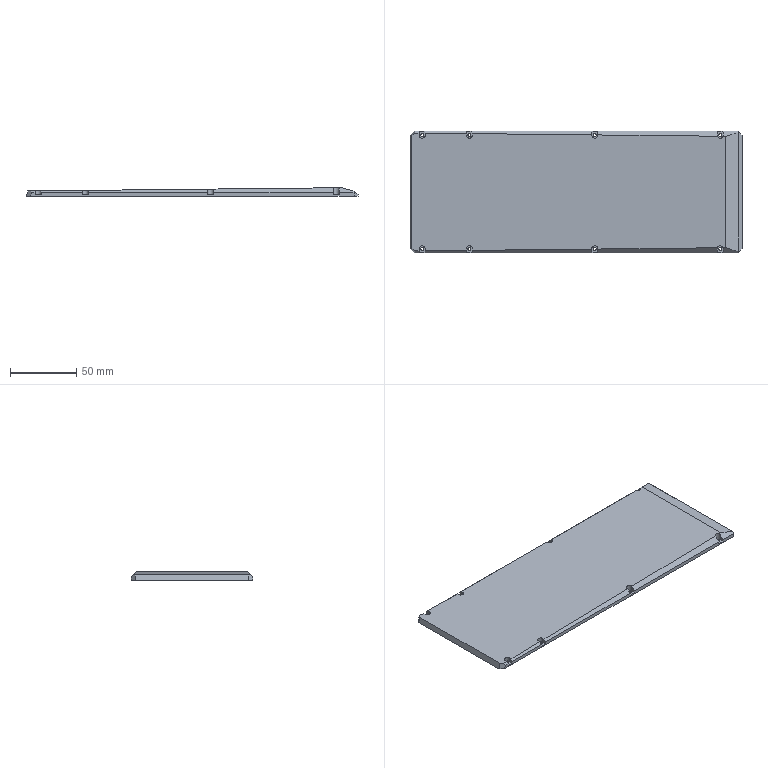CAM job | NX | 3-axis milling, drilling | part box 251.5 x 92 x 6.5 mm | stock box 260 x 100 x 10 mm
Tools:
number,name,description,diameter,corner_radius,flute_length,length,flutes
2,D2-6-D4-50-3T-ROUGH,D2-6-D4-50-3T-粗,2.0,0.0,6.0,7.0,2
0,D3-9-D4-50-3T-ROUGH,D3-9-D4-50-3T,3.0,0.0,9.0,10.0,3
0,D3-9-D4-50-3T-FINISH,D3-9-D4-50-3T-精,3.0,0.0,9.0,10.0,2
3,D6-18-D6-50-3T-FINISH,D6-18-D6-50-3T,6.0,0.0,18.0,50.0,3
1,D10-30-D10-75-3T-ROUGH,D10-30-D10-75-3T-粗,10.0,0.0,30.0,75.0,2
1,D12-36-D12-120-3TFINISH,D12-55-D12-120-3T,12.0,0.0,55.0,120.0,3
13,D50FACEMILL,D50面刀,50.0,0.0,30.0,30.0,4
11,D63FACEMILL,D63面刀,63.0,0.0,30.0,30.0,4
3,DRILLD1.84-11-D3-40,钻刀D1.84-11-D3-40,1.84,0.0,11.0,12.0,2
5,DRILLD2.4-35-61,钻刀D2.5-35-61,2.4,0.0,36.0,61.0,2
5,FORMTAPM2-12-D3-39,挤压M2-12-D3-39,2.0,0.0,12.5,14.5,2
4,CHAMFERD4-90DEG,倒角D4-90度,4.0,0.0,5.0,50.0,2
12,D4R0.5,Milling Tool-5 Parameters,4.0,0.5,50.0,75.0,2
Operations:
program,operation,operation_type,tool,method,geometry_group,spindle_rpm,surface_speed,feed_per_tooth,feed_cut,feed_plunge,cut_length_mm,path_length_mm,cut_time_min,machine_time_min
A1,PLANAR_MILL_4,PlanarMilling,D63FACEMILL,METHOD,A-G54,3500.0,692.0,0.0571,800.0,100.0,657.0,1096.483,0.8213,0.8652
A1,PLANAR_MILL,PlanarMilling,D10-30-D10-75-3T-ROUGH,METHOD,WORKPIECE_54,4500.0,141.0,0.1667,1500.0,100.0,8744.461,9081.313,5.83,5.863
A1,PLANAR_MILL_COPY_1,PlanarMilling,D10-30-D10-75-3T-ROUGH,METHOD,WORKPIECE_54,4500.0,141.0,0.1667,1500.0,100.0,4614.076,4868.443,3.076,3.102
A1,PLANAR_PROFILING,PlanarMilling,D10-30-D10-75-3T-ROUGH,METHOD,WORKPIECE_54,4500.0,141.0,0.1111,1000.0,100.0,5055.326,5144.065,5.055,5.064
A1,PLANAR_MILL_COPY_COPY,PlanarMilling,D6-18-D6-50-3T-FINISH,METHOD,WORKPIECE_54,4000.0,75.0,0.0667,800.0,100.0,69.184,577.146,0.0865,0.1373
A1,PLANAR_MILL_COPY_COPY_COPY_1,PlanarMilling,D6-18-D6-50-3T-FINISH,METHOD,WORKPIECE_54,4000.0,75.0,0.0667,800.0,100.0,34.592,216.179,0.0432,0.0614
A1,PLANAR_MILL_COPY,PlanarMilling,D6-18-D6-50-3T-FINISH,METHOD,WORKPIECE_54,4000.0,125.0,0.0667,800.0,100.0,1137.2,1194.6,1.421,1.427
A1,PLANAR_MILL_COPY_COPY_1,PlanarMilling,D6-18-D6-50-3T-FINISH,METHOD,WORKPIECE_54,4000.0,125.0,0.0667,800.0,100.0,2620.054,2682.454,3.275,3.281
A1,PLANAR_MILL_1,PlanarMilling,D6-18-D6-50-3T-FINISH,METHOD,WORKPIECE_54,4000.0,125.0,0.0667,800.0,100.0,710.995,780.995,0.8887,0.8957
A1,PLANAR_MILL_COPY_COPY_COPY,PlanarMilling,D6-18-D6-50-3T-FINISH,METHOD,WORKPIECE_54,4000.0,75.0,0.0667,800.0,100.0,448.283,510.683,0.5604,0.5666
A1,PLANAR_MILL_COPY_COPY_COPY_1_COPY,PlanarMilling,D6-18-D6-50-3T-FINISH,METHOD,WORKPIECE_54,4000.0,75.0,0.0667,800.0,100.0,216.283,275.683,0.2704,0.2763
A1,PLANAR_MILL_5,PlanarMilling,D6-18-D6-50-3T-FINISH,METHOD,A-G54,6500.0,122.0,0.041,800.0,100.0,740.395,1024.154,0.9255,0.9539
A1,PLANAR_MILL_5_COPY,PlanarMilling,D6-18-D6-50-3T-FINISH,METHOD,A-G54,6500.0,122.0,0.041,800.0,100.0,185.899,251.499,0.2324,0.2389
A1,平面铣倒角,PlanarMilling,CHAMFERD4-90DEG,METHOD,WORKPIECE_54,3500.0,43.0,0.1429,1000.0,100.0,585.85,641.85,0.5859,0.5915
A1,PLANAR_MILL_5_COPY_COPY,PlanarMilling,CHAMFERD4-90DEG,METHOD,A-G54,4500.0,56.0,0.0667,600.0,100.0,193.876,259.076,0.3231,0.3296
A1,平面铣倒角_COPY,PlanarMilling,CHAMFERD4-90DEG,METHOD,WORKPIECE_54,3500.0,43.0,0.1429,1000.0,100.0,81.284,139.684,0.0813,0.0871
A1,平面铣倒角_1,PlanarMilling,CHAMFERD4-90DEG,METHOD,WORKPIECE_54,3500.0,43.0,0.1429,1000.0,100.0,696.845,754.845,0.6968,0.7026
A1,DRILLING,Operation,CHAMFERD4-90DEG,METHOD,WORKPIECE_54,3000.0,37.0,0.025,150.0,0.0,34.0,1169.84,0.2267,0.3403
A1,DRILLING_COPY,Operation,DRILLD2.4-35-61,METHOD,WORKPIECE_54,3000.0,22.0,0.0333,200.0,0.0,72.0,1245.84,0.36,0.4774
B1,ADAPTIVE_MILLING,CavityMilling,D10-30-D10-75-3T-ROUGH,METHOD,WORKPIECE_55,6500.0,204.0,0.2308,3000.0,100.0,59868.173,68596.254,13.506,14.379
B1,CURVE_DRIVE_COPY,SurfaceContour,D4R0.5,METHOD,B-G55,6000.0,188.0,0.25,3000.0,100.0,20608.91,20984.951,6.87,6.907
B1,CURVE_DRIVE_COPY_COPY,SurfaceContour,D4R0.5,METHOD,B-G55,6000.0,188.0,0.25,3000.0,100.0,21012.824,22542.308,7.004,7.157
B1,CURVE_DRIVE_COPY_COPY_COPY,SurfaceContour,D4R0.5,METHOD,B-G55,6000.0,188.0,0.25,3000.0,100.0,473.306,685.412,0.1578,0.179
C1,FLOOR_FACING_1,VolumeBased25DMillingOperation,D50FACEMILL,METHOD,C-G56,3000.0,100.0,0.1178,800.0,100.0,930.818,984.718,1.163,1.169
C1,FLOOR_FACING_1_COPY,VolumeBased25DMillingOperation,D50FACEMILL,METHOD,C-G56,3000.0,100.0,0.1178,800.0,100.0,930.818,984.818,1.163,1.169
D1,PLANAR_MILL_3,PlanarMilling,D3-9-D4-50-3T-FINISH,METHOD,D-G57,3500.0,32.0,0.0857,600.0,100.0,128.137,863.618,0.2136,0.2871
G-G59,PLANAR_MILL_2,PlanarMilling,D3-9-D4-50-3T-ROUGH,METHOD,B-G55,5500.0,51.0,0.0606,1000.0,100.0,2886.053,4072.391,2.886,3.005
G-G59,CURVE_DRIVE,SurfaceContour,D4R0.5,METHOD,B-G55,6000.0,188.0,0.25,3000.0,100.0,158154.261,158211.004,52.718,52.724
FIXTURE1,FLOOR_FACING,VolumeBased25DMillingOperation,D12-36-D12-120-3TFINISH,METHOD,GZ1,4000.0,100.0,0.1178,2000.0,100.0,5241.465,5439.135,2.621,2.64
FIXTURE1,FLOOR_FACING_COPY,VolumeBased25DMillingOperation,D12-36-D12-120-3TFINISH,METHOD,GZ1,4000.0,100.0,0.1178,800.0,100.0,2680.896,2740.896,3.351,3.357
FIXTURE1,PLANAR_MILL_6_COPY_COPY,PlanarMilling,D2-6-D4-50-3T-ROUGH,METHOD,GZ1,4500.0,100.0,0.1178,600.0,100.0,672.376,2939.095,1.121,1.347
FIXTURE1,PLANAR_MILL_6_COPY_COPY_COPY,PlanarMilling,D2-6-D4-50-3T-ROUGH,METHOD,GZ1,4500.0,100.0,0.1178,600.0,100.0,96.054,759.554,0.1601,0.2264
FIXTURE1,DRILLING_1,Operation,CHAMFERD4-90DEG,METHOD,GZ1,2000.0,0.0,0.0,200.0,0.0,32.0,687.013,0.16,0.2255
FIXTURE1,DRILLING_1_COPY,Operation,DRILLD1.84-11-D3-40,METHOD,GZ1,2500.0,14.0,0.03,150.0,0.0,88.0,799.013,0.5867,0.6578
FIXTURE1,DRILLING_1_COPY_COPY,Operation,FORMTAPM2-12-D3-39,METHOD,GZ1,300.0,1.0,0.0007,0.4,0.0,72.0,767.013,180.0,180.07
FIXTURE1,PLANAR_MILL_6_COPY,PlanarMilling,D12-36-D12-120-3TFINISH,METHOD,GZ1,4000.0,100.0,0.1178,800.0,100.0,649.683,709.683,0.8121,0.8181